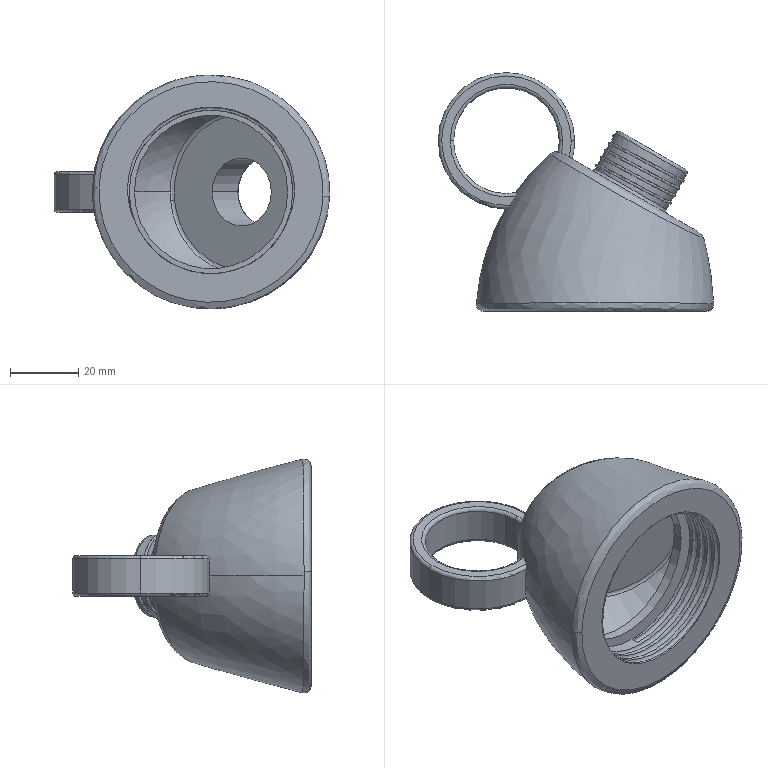Part | SolidWorks | features Fillet 6, ICE 6, Helix 3, Sculpt 3, BaseBody 2, DeleteBody 2, Shell 2, Sweep 2, Blend 1, CombineBodies 1, RefAxis 1, Revolution 1, Split 1, SweepCut 1 | 1 solid | 71 faces | volume 42734 mm3 | cylinder 28 | spline 16 | torus 16 | plane 11 | commonest cylinder face diameters 24 x10 48 x8 31 x3 40 x3 20 x2 45 x2